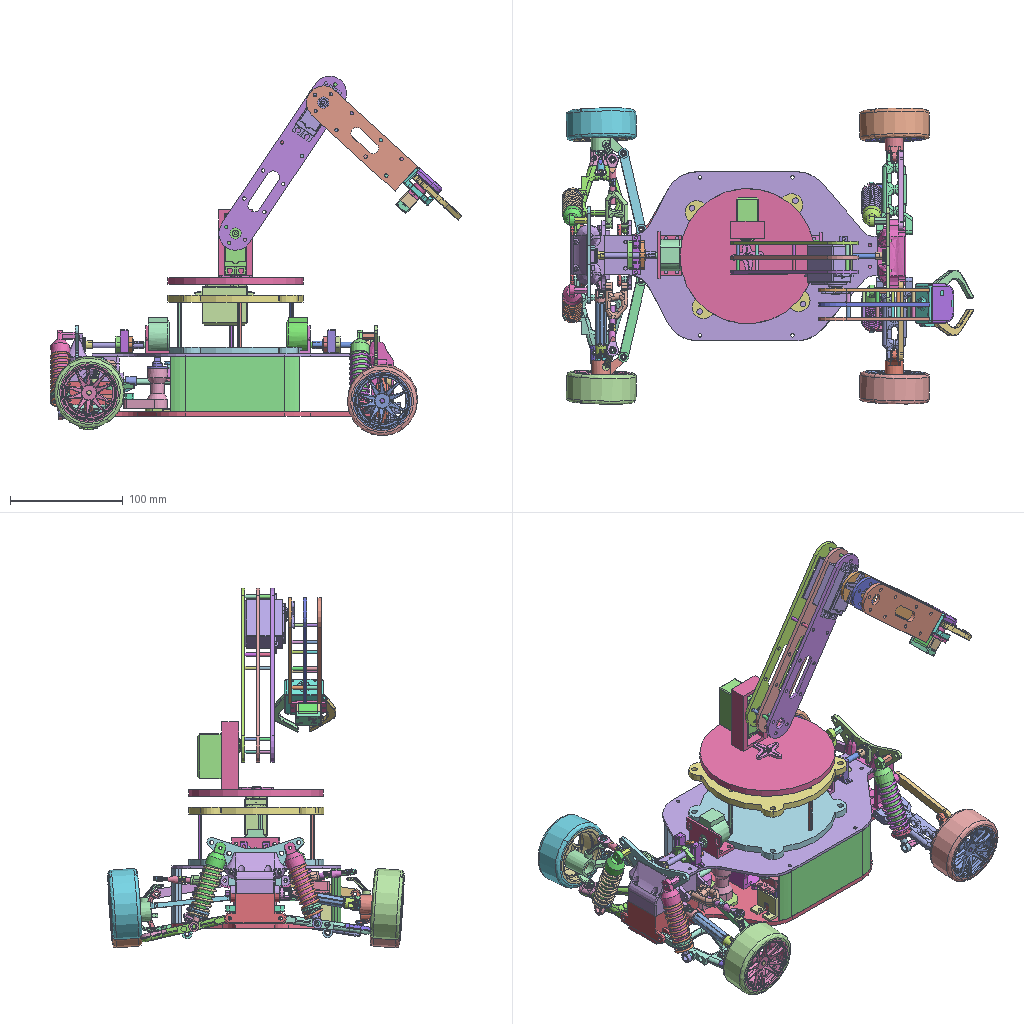Assembly | STEP file | 148 different items | 148 placed | box 365 x 263 x 319 mm
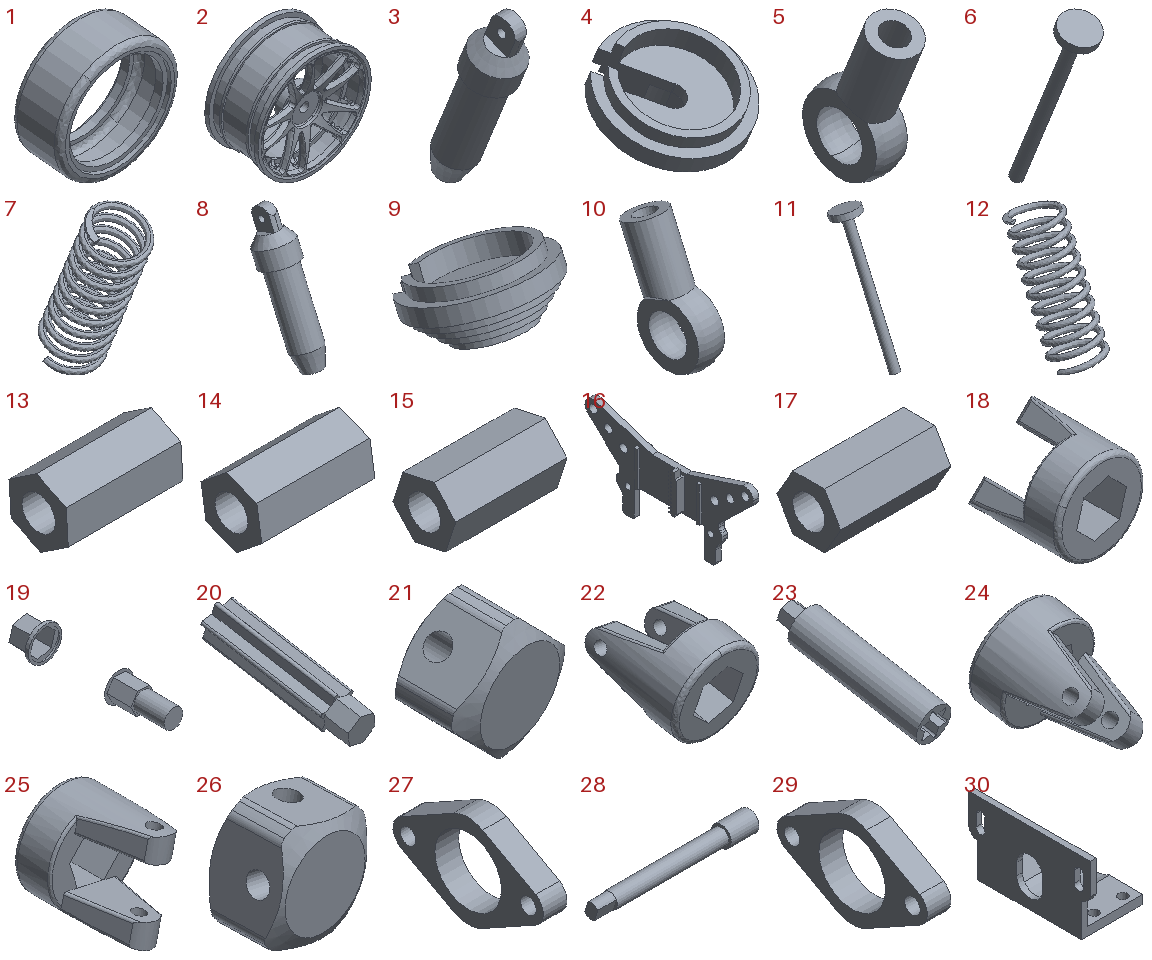Parts list (item | name | quantity | parent item | size | volume):
1 | PNEU | x1 | in JR29_2 | 62.467 x 30.182 x 63.29 mm | 18321 mm3
2 | jante JR29 | x1 | in JR29_2 | 53.113 x 29.9 x 54.23 mm | 11757 mm3
3 | Cut-Extrude2 | x1 | in _115-006 | 16.64 x 30.437 x 60.503 mm | 5800 mm3
4 | Cut-Extrude7 | x1 | in _115-003 | 18 x 17.564 x 12.214 mm | 867.182 mm3
5 | _.0mm Dowel Hole1 | x1 | in _115-001 | 5.5 x 12.284 x 18.097 mm | 294.625 mm3
6 | Revolve1 | x1 | in _115-004 | 9.4 x 23.118 x 45.968 mm | 456.882 mm3
7 | Ci_cie powierzchni_3 | x1 | in _120-006 | 18 x 31.651 x 49.627 mm | 1562 mm3
8 | Cut-Extrude2 | x1 | in _115-006 | 16.64 x 32.155 x 59.897 mm | 5800 mm3
9 | Cut-Extrude7 | x1 | in _115-003 | 18 x 17.404 x 12.495 mm | 867.182 mm3
10 | _.0mm Dowel Hole1 | x1 | in _115-001 | 5.5 x 12.651 x 18.014 mm | 294.626 mm3
11 | Revolve1 | x1 | in _115-004 | 9.4 x 24.478 x 45.558 mm | 456.882 mm3
12 | Ci_cie powierzchni_3 | x1 | in _120-006 | 18 x 34.556 x 45.056 mm | 1562 mm3
13 | Dodanie-wyci_gni_cie1_8 | x1 | in dystanse amortyzatora | 11 x 5.689 x 6.325 mm | 198.638 mm3
14 | Dodanie-wyci_gni_cie1_8 | x1 | in dystanse amortyzatora | 11 x 5.919 x 6.26 mm | 198.638 mm3
15 | Dodanie-wyci_gni_cie1_8 | x1 | in dystanse amortyzatora | 11 x 6.193 x 6.041 mm | 198.638 mm3
16 | Dodanie-wyci_gni_cie4_3 | x1 | in _400-008 | 8.15 x 85.559 x 42.443 mm | 4763 mm3
17 | Dodanie-wyci_gni_cie1_8 | x1 | in dystanse amortyzatora | 11 x 6.339 x 5.502 mm | 198.638 mm3
18 | Wytnij-wyci_gni_cie1_8 | x1 | in _151-004 | 10.019 x 11.057 x 10.028 mm | 351.853 mm3
19 | Przeci_cie1[1] | x1 | in _151-002 | 7.004 x 31.35 x 7.006 mm | 710.625 mm3
20 | Dodanie-wyci_gni_cie2_4 | x1 | in _151-005 | 7.193 x 30.668 x 11.467 mm | 797.649 mm3
21 | Wytnij-wyci_gni_cie2_4 | x1 | in _151-003 | 6.818 x 4.485 x 6.828 mm | 88.126 mm3
22 | Wytnij-wyci_gni_cie1_8 | x1 | in _151-004 | 10.007 x 11.818 x 10.415 mm | 351.853 mm3
23 | Dodanie-wyci_gni_cie3 | x1 | in _151-006 | 9.523 x 41.689 x 15.416 mm | 1560 mm3
24 | Wytnij-wyci_gni_cie1_8 | x1 | in _151-004 | 10.002 x 12.22 x 10.913 mm | 351.853 mm3
25 | Wytnij-wyci_gni_cie1_8 | x1 | in _151-004 | 10 x 11 x 10 mm | 351.853 mm3
26 | Wytnij-wyci_gni_cie2_4 | x1 | in _151-003 | 5.85 x 4.13 x 6.16 mm | 88.126 mm3
27 | Dodanie-wyci_gni_cie1_6 | x1 | in _400-005 | 3.95 x 25 x 15.427 mm | 542.296 mm3
28 | Dodanie-wyci_gni_cie4_1 | x1 | in _400-003 | 51 x 6.5 x 6.5 mm | 982.022 mm3
29 | Dodanie-wyci_gni_cie1_6 | x1 | in _400-005 | 3.95 x 25 x 15.427 mm | 542.296 mm3
30 | Wytnij-wyci_gni_cie6_2 | x1 | in _400-002 | 21.259 x 42 x 25 mm | 3415 mm3
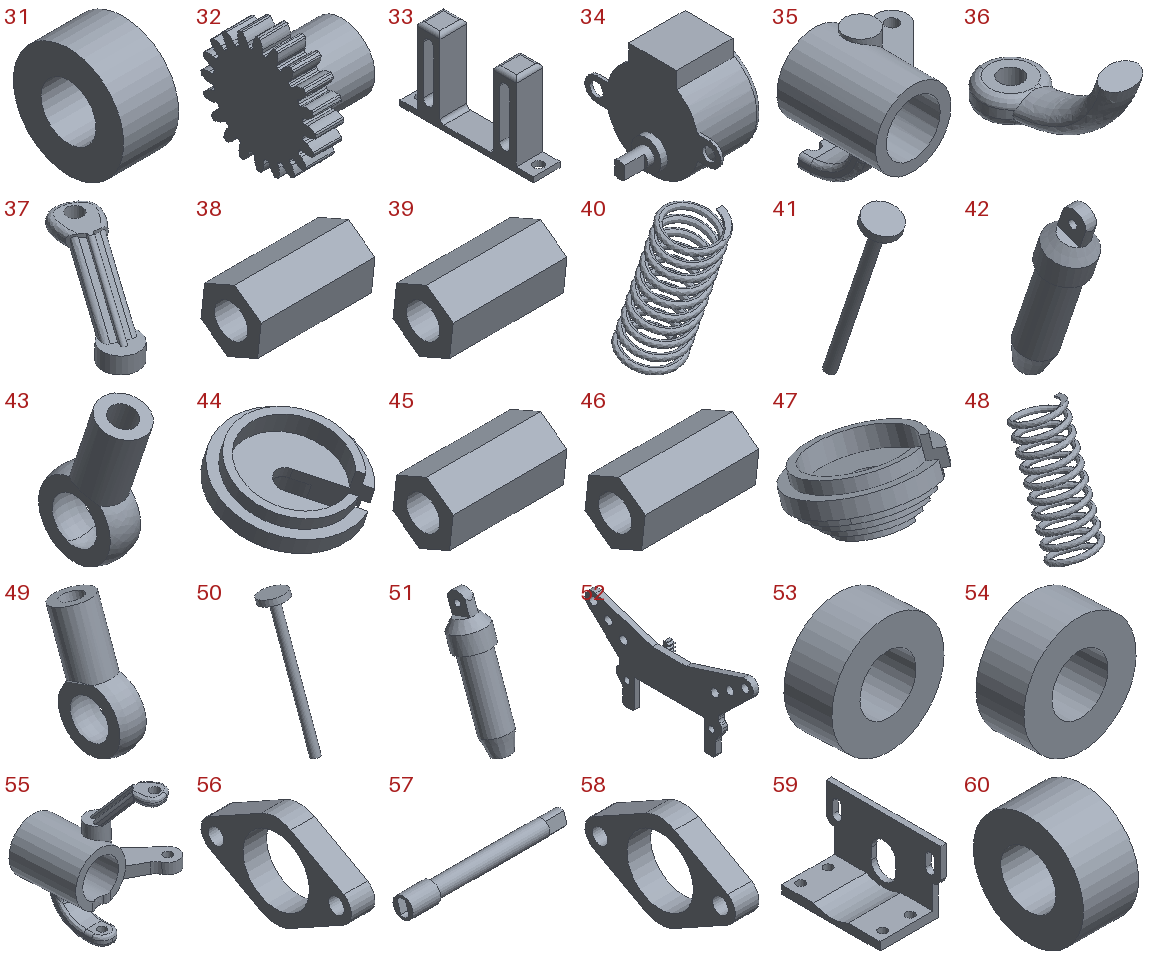31 | Dodanie-wyci_gni_cie1_7 | x1 | in _400-007 | 5 x 10 x 10 mm | 294.524 mm3
32 | Wytnij-wyci_gni_cie1_7 | x1 | in _400-006 | 9 x 12.32 x 12.32 mm | 463.728 mm3
33 | Wytnij-wyci_gni_cie4 | x1 | in _400-004 | 7 x 35 x 21.379 mm | 1461 mm3
34 | Wytnij-wyci_gni_cie1_6 | x1 | in _400-001 | 29 x 41 x 31 mm | 12849 mm3
35 | Zaokr_glenie5_1 | x1 | in _140-001-lewa | 32.058 x 28.351 x 26.679 mm | 3338 mm3
36 | Wytnij-wyci_gni_cie10 | x1 | in _140-001-lewa | 7.005 x 17.81 x 9.853 mm | 233.546 mm3
37 | - | x1 | in _140-001-lewa | 12.902 x 21.037 x 15.015 mm | 400.583 mm3
38 | Dodanie-wyci_gni_cie1_8 | x1 | in dystanse amortyzatora | 11 x 5.805 x 6.301 mm | 198.638 mm3
39 | Dodanie-wyci_gni_cie1_8 | x1 | in dystanse amortyzatora | 11 x 5.805 x 6.301 mm | 198.638 mm3
40 | Ci_cie powierzchni_3 | x1 | in _120-006 | 18 x 31.486 x 45.126 mm | 1562 mm3
41 | Revolve1 | x1 | in _115-004 | 9.4 x 20.928 x 46.51 mm | 456.882 mm3
42 | Cut-Extrude2 | x1 | in _115-006 | 16.64 x 27.67 x 61.336 mm | 5800 mm3
43 | _.0mm Dowel Hole1 | x1 | in _115-001 | 5.5 x 11.691 x 18.199 mm | 294.626 mm3
44 | Cut-Extrude7 | x1 | in _115-003 | 18 x 17.777 x 11.744 mm | 867.182 mm3
45 | Dodanie-wyci_gni_cie1_8 | x1 | in dystanse amortyzatora | 11 x 5.805 x 6.301 mm | 198.638 mm3
46 | Dodanie-wyci_gni_cie1_8 | x1 | in dystanse amortyzatora | 11 x 5.805 x 6.301 mm | 198.638 mm3
47 | Cut-Extrude7 | x1 | in _115-003 | 18 x 17.702 x 11.925 mm | 867.182 mm3
48 | Ci_cie powierzchni_3 | x1 | in _120-006 | 18 x 30.619 x 49.676 mm | 1562 mm3
49 | _.0mm Dowel Hole1 | x1 | in _115-001 | 5.5 x 11.917 x 18.165 mm | 294.625 mm3
50 | Revolve1 | x1 | in _115-004 | 9.4 x 21.762 x 46.32 mm | 456.882 mm3
51 | Cut-Extrude2 | x1 | in _115-006 | 16.64 x 28.724 x 61.039 mm | 5800 mm3
52 | Zapas-_111-007-1 | x1 | in _400-009.1 | 6.85 x 85.559 x 42.443 mm | 4712 mm3
53 | Dodanie-wyci_gni_cie1_3 | x1 | in _140-002 | 12.066 x 5.461 x 12.174 mm | 424.115 mm3
54 | Dodanie-wyci_gni_cie1_3 | x1 | in _140-002 | 12.066 x 5.461 x 12.174 mm | 424.115 mm3
55 | Zaokr_glenie5 | x1 | in _140-001-prawa | 32.405 x 33.388 x 41.862 mm | 3783 mm3
56 | Dodanie-wyci_gni_cie1_6 | x1 | in _400-005 | 3.95 x 25 x 15.427 mm | 542.296 mm3
57 | Dodanie-wyci_gni_cie4_1 | x1 | in _400-003 | 51 x 6.5 x 6.5 mm | 982.022 mm3
58 | Dodanie-wyci_gni_cie1_6 | x1 | in _400-005 | 3.95 x 25 x 15.427 mm | 542.296 mm3
59 | Wytnij-wyci_gni_cie6_2 | x1 | in _400-002 | 21.259 x 42 x 25 mm | 3415 mm3
60 | Dodanie-wyci_gni_cie1_7 | x1 | in _400-007 | 5 x 10 x 10 mm | 294.524 mm3
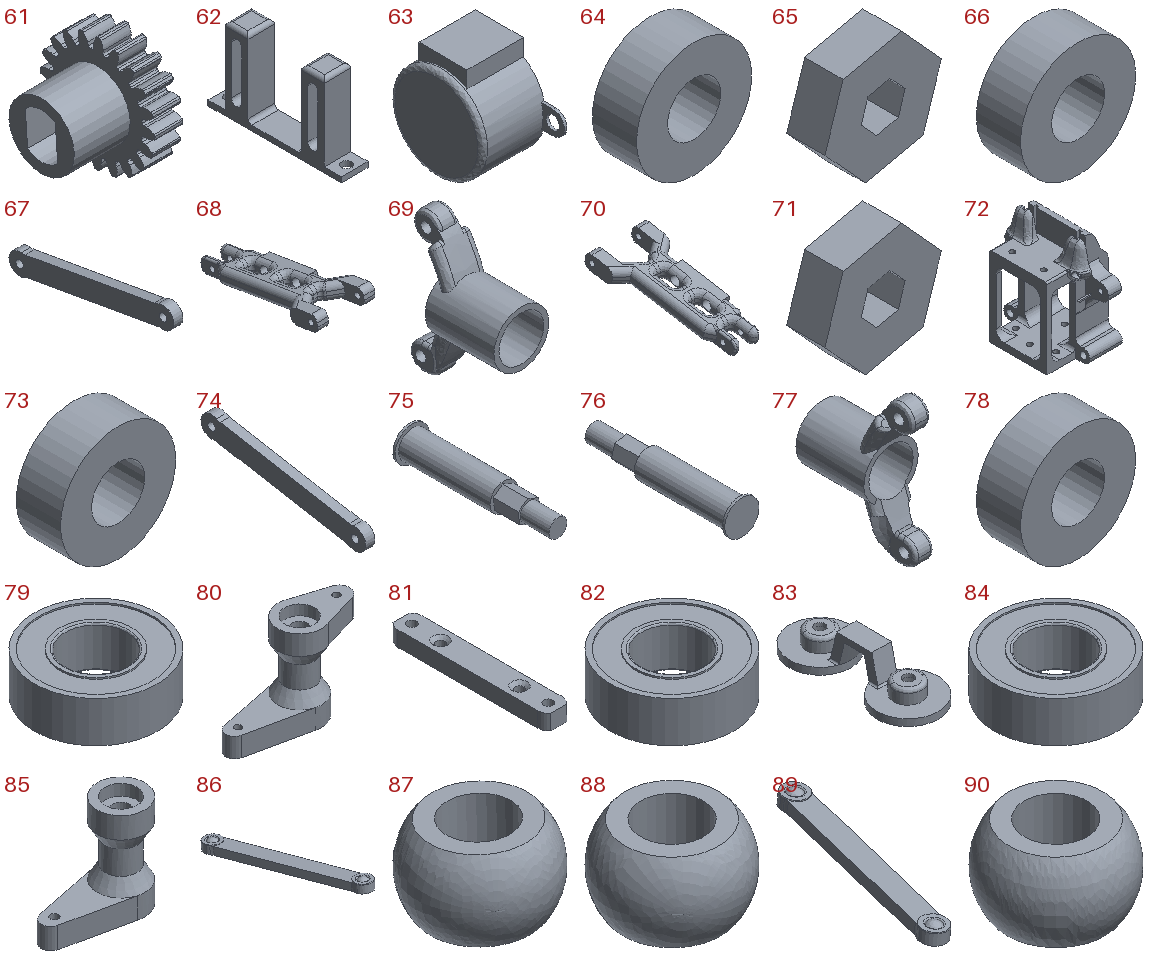61 | Wytnij-wyci_gni_cie1_7 | x1 | in _400-006 | 9 x 12.32 x 12.32 mm | 463.728 mm3
62 | Wytnij-wyci_gni_cie4 | x1 | in _400-004 | 7 x 35 x 21.379 mm | 1461 mm3
63 | Wytnij-wyci_gni_cie1_6 | x1 | in _400-001 | 29 x 41 x 31 mm | 12849 mm3
64 | Dodanie-wyci_gni_cie1_4 | x1 | in _200-006 | 13 x 5.005 x 13.002 mm | 522.29 mm3
65 | Dodanie-wyci_gni_cie1_5 | x1 | in _150-003 | 13.678 x 4.505 x 13.341 mm | 491.011 mm3
66 | Dodanie-wyci_gni_cie1_4 | x1 | in _200-006 | 13 x 5.005 x 13.002 mm | 522.29 mm3
67 | Dodanie-wyci_gni_cie2_2 | x1 | in _200-003 | 4 x 70.047 x 19.826 mm | 2190 mm3
68 | Wytnij-wyci_gni_cie2_2 | x1 | in _200-002 | 32 x 74.835 x 19.276 mm | 7840 mm3
69 | Wytnij-wyci_gni_cie8 | x1 | in _200-004 | 16 x 29.947 x 40.939 mm | 2434 mm3
70 | Wytnij-wyci_gni_cie2_2 | x1 | in _200-002 | 32 x 74.835 x 19.276 mm | 7840 mm3
71 | Dodanie-wyci_gni_cie1_5 | x1 | in _150-003 | 13.678 x 4.505 x 13.341 mm | 491.011 mm3
72 | Lustro3 | x1 | in _200-001 | 37.601 x 63.709 x 62.254 mm | 29031 mm3
73 | Dodanie-wyci_gni_cie1_4 | x1 | in _200-006 | 13 x 5.005 x 13.002 mm | 522.29 mm3
74 | Dodanie-wyci_gni_cie2_2 | x1 | in _200-003 | 4 x 70.047 x 19.826 mm | 2190 mm3
75 | Dodanie-wyci_gni_cie4_2 | x1 | in _200-005 | 7.5 x 32.302 x 7.5 mm | 765.405 mm3
76 | Dodanie-wyci_gni_cie4_2 | x1 | in _200-005 | 7.5 x 32.302 x 7.5 mm | 765.405 mm3
77 | Wytnij-wyci_gni_cie8 | x1 | in _200-004 | 16 x 29.947 x 40.939 mm | 2434 mm3
78 | Dodanie-wyci_gni_cie1_4 | x1 | in _200-006 | 13 x 5.005 x 13.002 mm | 522.29 mm3
79 | Zapas-OpenRC Truggy HSPr v2. v55-1 | x1 | in _131-003 | 12 x 12 x 4 mm | 322.133 mm3
80 | Dodanie-wyci_gni_cie2 | x1 | in _131-002 | 50.275 x 17.999 x 35 mm | 7787 mm3
81 | Wytnij-wyci_gni_cie1_1 | x1 | in _131-006 | 8 x 52 x 5 mm | 1902 mm3
82 | Zapas-OpenRC Truggy HSPr v2. v55-1 | x1 | in _131-003 | 12 x 12 x 4 mm | 322.133 mm3
83 | Wytnij-wyci_gni_cie3_1 | x1 | in _131-008 | 18.204 x 43.999 x 10 mm | 1454 mm3
84 | Zapas-OpenRC Truggy HSPr v2. v55-1 | x1 | in _131-003 | 12 x 12 x 4 mm | 322.133 mm3
85 | Dodanie-wyci_gni_cie1_2 | x1 | in _131-005 | 38.999 x 17.999 x 35 mm | 6844 mm3
86 | Zaokr_glenie2 | x1 | in _131-007 | 24.844 x 77.037 x 13.475 mm | 2577 mm3
87 | Wytnij-wyci_gni_cie1_2 | x1 | in kulka przegubu sterowania | - | 61.693 mm3
88 | Wytnij-wyci_gni_cie1_2 | x1 | in kulka przegubu sterowania | - | 61.693 mm3
89 | Zaokr_glenie2 | x1 | in _131-007 | 25.053 x 77.12 x 7.399 mm | 2577 mm3
90 | Wytnij-wyci_gni_cie1_2 | x1 | in kulka przegubu sterowania | - | 61.693 mm3
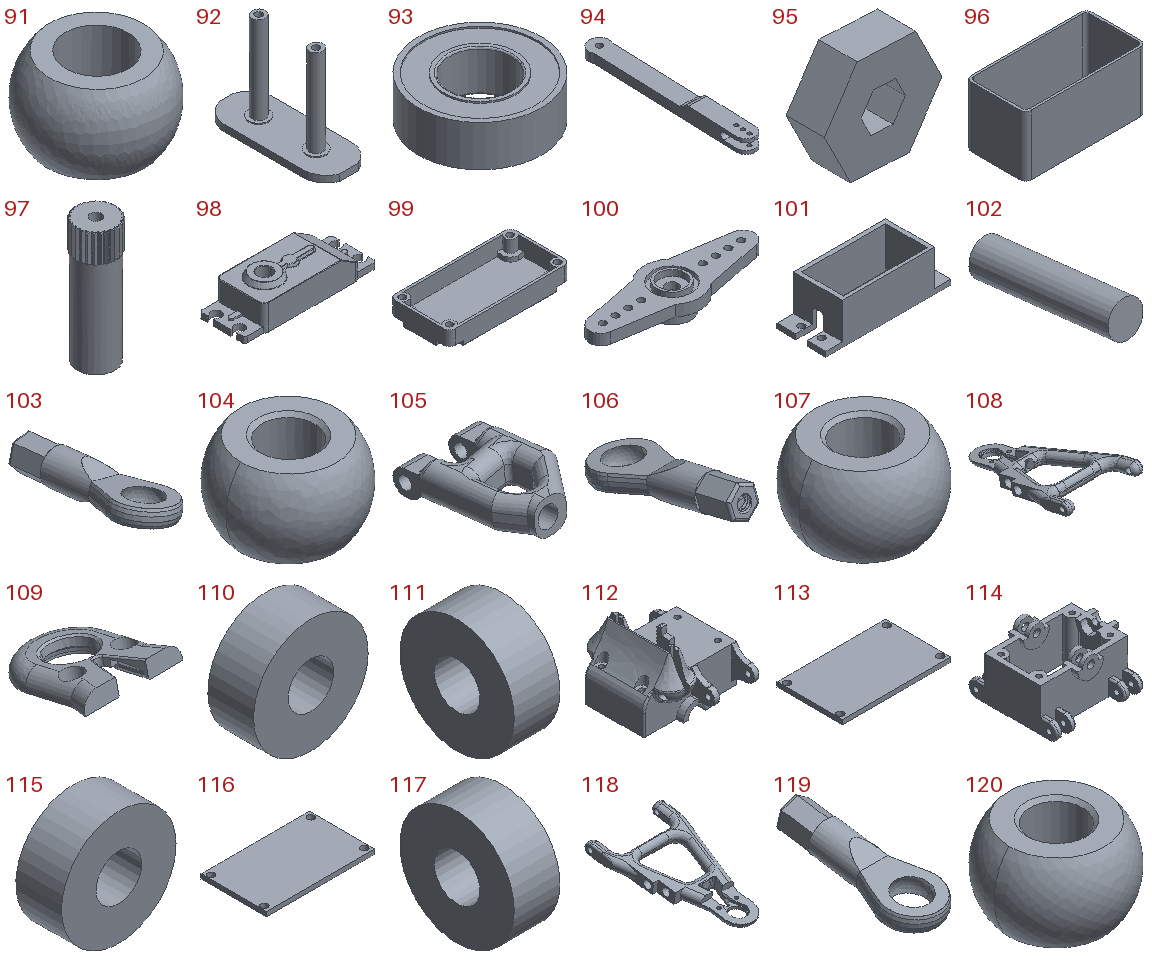91 | Wytnij-wyci_gni_cie1_2 | x1 | in kulka przegubu sterowania | - | 61.693 mm3
92 | Wytnij-wyci_gni_cie1 | x1 | in _131-004 | 21.875 x 55.54 x 43 mm | 5051 mm3
93 | Zapas-OpenRC Truggy HSPr v2. v55-1 | x1 | in _131-003 | 12 x 12 x 4 mm | 322.133 mm3
94 | Wytnij-wyci_gni_cie3 | x1 | in _131-001 | 10.909 x 75.957 x 6 mm | 2529 mm3
95 | Dodanie-wyci_gni_cie1_5 | x1 | in _150-003 | 14.005 x 4.648 x 12.539 mm | 491.011 mm3
96 | Zapas-OpenRC Truggy HSPr v2. v55-3 | x1 | in _132-001 | 41 x 20.4 x 20.5 mm | 1916 mm3
97 | Zapas-OpenRC Truggy HSPr v2. v55-4 | x1 | in _132-001 | 5.799 x 5.767 x 17.5 mm | 382.741 mm3
98 | Zapas-OpenRC Truggy HSPr v2. v55-2 | x1 | in _132-001 | 56 x 20.4 x 13 mm | 9258 mm3
99 | Zapas-OpenRC Truggy HSPr v2. v55-1_1 | x1 | in 99 | - | -
100 | Zapas-OpenRC Truggy HSPr v2. v55-1_2 | x1 | in _132-004 | 38.395 x 12.8 x 5.95 mm | 788.17 mm3
101 | Wytnij-wyci_gni_cie2_3 | x1 | in _132-003 | 60.8 x 23.8 x 20 mm | 5414 mm3
102 | Dodanie-wyci_gni_cie1_1 | x1 | in _114-003 | 5 x 20.432 x 7.194 mm | 392.699 mm3
103 | Zapas-_112-004-1_2 | x1 | in Zapas-_112-004-1 | - | -
104 | Spare ball joint-1 | x1 | in Ball joint-ball | 7 x 7 x 4.494 mm | 116.194 mm3
105 | Wytnij-wyci_gni_cie2 | x1 | in _114-000 | 20 x 33.148 x 11.306 mm | 2601 mm3
106 | Zapas-_112-004-1_2 | x1 | in Zapas-_112-004-1 | - | -
107 | Spare ball joint-1 | x1 | in Ball joint-ball | 7 x 7 x 4.635 mm | 116.194 mm3
108 | Wytnij-wyci_gni_cie6_1 | x1 | in _112-003 | 48 x 82.899 x 24.651 mm | 7377 mm3
109 | - | x1 | in _112-001 | 21.033 x 23.076 x 8.696 mm | 790.702 mm3
110 | Dodanie-wyci_gni_cie1 | x1 | in _111-004 | 10 x 4 x 10 mm | 263.894 mm3
111 | Dodanie-wyci_gni_cie1 | x1 | in _111-004 | 4 x 10 x 10 mm | 263.894 mm3
112 | Wytnij-wyci_gni_cie6 | x1 | in _111-001 | 58 x 61.646 x 42.232 mm | 26812 mm3
113 | Wytnij-wyci_gni_cie8[2] | x1 | in _111-000 | 48 x 29 x 2 mm | 2727 mm3
114 | - | x1 | in _111-000 | 58 x 55 x 32 mm | 19800 mm3
115 | Dodanie-wyci_gni_cie1 | x1 | in _111-004 | 10 x 4 x 10 mm | 263.894 mm3
116 | Zapas-_111-000-1 | x1 | in _111-002 | 48 x 29 x 2 mm | 2727 mm3
117 | Dodanie-wyci_gni_cie1 | x1 | in _111-004 | 4 x 10 x 10 mm | 263.894 mm3
118 | Zaokr_glenie6 | x1 | in _112-002 | 48 x 84.201 x 17.884 mm | 7214 mm3
119 | Zapas-_112-004-1_2 | x1 | in Zapas-_112-004-1 | - | -
120 | Spare ball joint-1 | x1 | in Ball joint-ball | 7 x 7 x 4.494 mm | 116.194 mm3
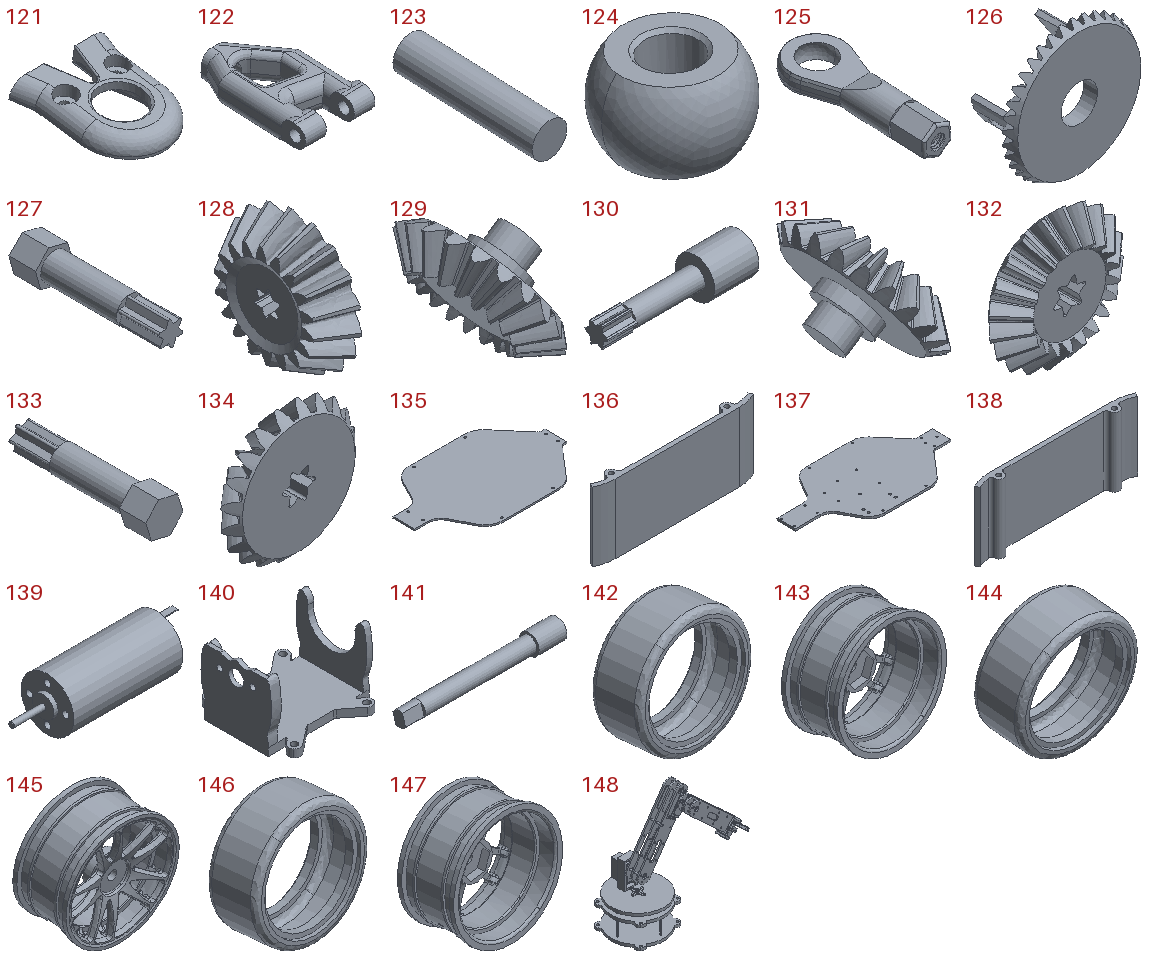121 | - | x1 | in _112-001 | 21.033 x 23.36 x 6.725 mm | 790.702 mm3
122 | Wytnij-wyci_gni_cie2 | x1 | in _114-000 | 20 x 33.189 x 9.079 mm | 2601 mm3
123 | Dodanie-wyci_gni_cie1_1 | x1 | in _114-003 | 5 x 20.198 x 5.864 mm | 392.699 mm3
124 | Spare ball joint-1 | x1 | in Ball joint-ball | 7 x 7 x 4.635 mm | 116.194 mm3
125 | Zapas-_112-004-1_2 | x1 | in Zapas-_112-004-1 | - | -
126 | Zaokr_glenie1 | x1 | in _152-003 | 36.885 x 17.8 x 36.885 mm | 3718 mm3
127 | Zapas-_150-001-1 | x1 | in _151-001 p1 | 5.61 x 21.6 x 5.588 mm | 281.637 mm3
128 | Wytnij-wyci_gni_cie1_3 | x1 | in _150-004(obci_te z_by) | 6 x 19.721 x 19.771 mm | 1055 mm3
129 | Dodanie-wyci_gni_cie2_1 | x1 | in _152-002 | 10.182 x 16.004 x 13.419 mm | 470.763 mm3
130 | Wytnij-wyci_gni_cie5 | x1 | in _150-002 | 29 x 8 x 8 mm | 614.096 mm3
131 | Dodanie-wyci_gni_cie2_1 | x1 | in _152-002 | 10.186 x 16.022 x 13.435 mm | 470.763 mm3
132 | Wytnij-wyci_gni_cie2_1 | x1 | in _152-001 | 15.995 x 3.782 x 15.995 mm | 380.18 mm3
133 | Zapas-_150-001-1 | x1 | in _151-001 p1 | 5.649 x 21.6 x 5.542 mm | 281.637 mm3
134 | Wytnij-wyci_gni_cie2_1 | x1 | in _152-001 | 15.956 x 3.782 x 15.956 mm | 380.18 mm3
135 | Dodanie-wyci_gni_cie2_3 | x1 | in _310-003SLDPRT | 242.308 x 150 x 2.5 mm | 66669 mm3
136 | Zaokr_glenie1_1 | x1 | in _310-004SLDPRT | 114.379 x 8.512 x 49 mm | 19491 mm3
137 | Wytnij-wyci_gni_cie1_5 | x1 | in _310-001 | 296.104 x 150 x 4 mm | 113905 mm3
138 | Zaokr_glenie1_1 | x1 | in _310-004SLDPRT | 114.379 x 8.512 x 49 mm | 19491 mm3
139 | Wytnij-wyci_gni_cie1_4 | x1 | in _153-001 | 75 x 24.6 x 24.6 mm | 24401 mm3
140 | Dodanie-wyci_gni_cie4 | x1 | in _153-003 | 52 x 49.249 x 34.708 mm | 13507 mm3
141 | Dodanie-wyci_gni_cie4_1 | x1 | in _400-003 | 51 x 6.5 x 6.5 mm | 982.022 mm3
142 | PNEU_ Mirror _1 | x1 | in JR29_3_ Mirror | 62.467 x 30.182 x 63.29 mm | 18324 mm3
143 | rim JR29_ Mirror _1 | x1 | in JR29_3_ Mirror | 53.113 x 29.9 x 54.23 mm | 11755 mm3
144 | PNEU | x1 | in JR29_2 | 62.467 x 30.182 x 63.29 mm | 18321 mm3
145 | jante JR29 | x1 | in JR29_2 | 53.113 x 29.9 x 54.23 mm | 11757 mm3
146 | PNEU_ Mirror | x1 | in JR29_2_ Mirror | 62.467 x 30.182 x 63.29 mm | 18324 mm3
147 | rim JR29_ Mirror | x1 | in JR29_2_ Mirror | 53.113 x 29.9 x 54.23 mm | 11755 mm3
148 | Assem1 | x1 | in Wheeled robot | 260.751 x 130.76 x 246.419 mm | 394553 mm3
Placements (level | parent | child | x y z in mm | rotation matrix by rows), first 269 of 321 lines:
1 | root | Frame drive system | 0.0 0.0 0.0 | 1 0 0 0 1 0 0 0 1
2 | Frame drive system | JR29_2 | 0.0 0.0 0.0 | 1 0 0 0 1 0 0 0 1
3 | JR29_2 | PNEU | 0.0 0.0 0.0 | 1 0 0 0 1 0 0 0 1
3 | JR29_2 | jante JR29 | 0.0 0.0 0.0 | 1 0 0 0 1 0 0 0 1
2 | Frame drive system | 000-000_1 | 0.0 0.0 0.0 | 1 0 0 0 1 0 0 0 1
3 | 000-000_1 | _122-000 | 0.0 0.0 0.0 | 1 0 0 0 1 0 0 0 1
4 | _122-000 | _120-000_2 | 0.0 0.0 0.0 | 1 0 0 0 1 0 0 0 1
5 | _120-000_2 | _115-006 | 0.0 0.0 0.0 | 1 0 0 0 1 0 0 0 1
6 | _115-006 | Cut-Extrude2 | 0.0 0.0 0.0 | 1 0 0 0 1 0 0 0 1
5 | _120-000_2 | _115-003 | 0.0 0.0 0.0 | 1 0 0 0 1 0 0 0 1
6 | _115-003 | Cut-Extrude7 | 0.0 0.0 0.0 | 1 0 0 0 1 0 0 0 1
5 | _120-000_2 | _115-001 | 0.0 0.0 0.0 | 1 0 0 0 1 0 0 0 1
6 | _115-001 | _.0mm Dowel Hole1 | 0.0 0.0 0.0 | 1 0 0 0 1 0 0 0 1
5 | _120-000_2 | _115-004 | 0.0 0.0 0.0 | 1 0 0 0 1 0 0 0 1
6 | _115-004 | Revolve1 | 0.0 0.0 0.0 | 1 0 0 0 1 0 0 0 1
5 | _120-000_2 | _120-006 | 0.0 0.0 0.0 | 1 0 0 0 1 0 0 0 1
6 | _120-006 | Ci_cie powierzchni_3 | 0.0 0.0 0.0 | 1 0 0 0 1 0 0 0 1
4 | _122-000 | _120-000_2 | 0.0 0.0 0.0 | 1 0 0 0 1 0 0 0 1
5 | _120-000_2 | _115-006 | 0.0 0.0 0.0 | 1 0 0 0 1 0 0 0 1
6 | _115-006 | Cut-Extrude2 | 0.0 0.0 0.0 | 1 0 0 0 1 0 0 0 1
5 | _120-000_2 | _115-003 | 0.0 0.0 0.0 | 1 0 0 0 1 0 0 0 1
6 | _115-003 | Cut-Extrude7 | 0.0 0.0 0.0 | 1 0 0 0 1 0 0 0 1
5 | _120-000_2 | _115-001 | 0.0 0.0 0.0 | 1 0 0 0 1 0 0 0 1
6 | _115-001 | _.0mm Dowel Hole1 | 0.0 0.0 0.0 | 1 0 0 0 1 0 0 0 1
5 | _120-000_2 | _115-004 | 0.0 0.0 0.0 | 1 0 0 0 1 0 0 0 1
6 | _115-004 | Revolve1 | 0.0 0.0 0.0 | 1 0 0 0 1 0 0 0 1
5 | _120-000_2 | _120-006 | 0.0 0.0 0.0 | 1 0 0 0 1 0 0 0 1
6 | _120-006 | Ci_cie powierzchni_3 | 0.0 0.0 0.0 | 1 0 0 0 1 0 0 0 1
4 | _122-000 | dystanse amortyzatora | 0.0 0.0 0.0 | 1 0 0 0 1 0 0 0 1
5 | dystanse amortyzatora | Dodanie-wyci_gni_cie1_8 | 0.0 0.0 0.0 | 1 0 0 0 1 0 0 0 1
4 | _122-000 | dystanse amortyzatora | 0.0 0.0 0.0 | 1 0 0 0 1 0 0 0 1
5 | dystanse amortyzatora | Dodanie-wyci_gni_cie1_8 | 0.0 0.0 0.0 | 1 0 0 0 1 0 0 0 1
4 | _122-000 | dystanse amortyzatora | 0.0 0.0 0.0 | 1 0 0 0 1 0 0 0 1
5 | dystanse amortyzatora | Dodanie-wyci_gni_cie1_8 | 0.0 0.0 0.0 | 1 0 0 0 1 0 0 0 1
4 | _122-000 | _400-008 | 0.0 0.0 0.0 | 1 0 0 0 1 0 0 0 1
5 | _400-008 | Dodanie-wyci_gni_cie4_3 | 0.0 0.0 0.0 | 1 0 0 0 1 0 0 0 1
4 | _122-000 | dystanse amortyzatora | 0.0 0.0 0.0 | 1 0 0 0 1 0 0 0 1
5 | dystanse amortyzatora | Dodanie-wyci_gni_cie1_8 | 0.0 0.0 0.0 | 1 0 0 0 1 0 0 0 1
3 | 000-000_1 | _151-000 | 0.0 0.0 0.0 | 1 0 0 0 1 0 0 0 1
4 | _151-000 | _151-004 | 0.0 0.0 0.0 | 1 0 0 0 1 0 0 0 1
5 | _151-004 | Wytnij-wyci_gni_cie1_8 | 0.0 0.0 0.0 | 1 0 0 0 1 0 0 0 1
4 | _151-000 | _151-002 | 0.0 0.0 0.0 | 1 0 0 0 1 0 0 0 1
5 | _151-002 | Przeci_cie1[1] | 0.0 0.0 0.0 | 1 0 0 0 1 0 0 0 1
4 | _151-000 | _151-005 | 0.0 0.0 0.0 | 1 0 0 0 1 0 0 0 1
5 | _151-005 | Dodanie-wyci_gni_cie2_4 | 0.0 0.0 0.0 | 1 0 0 0 1 0 0 0 1
4 | _151-000 | _151-003 | 0.0 0.0 0.0 | 1 0 0 0 1 0 0 0 1
5 | _151-003 | Wytnij-wyci_gni_cie2_4 | 0.0 0.0 0.0 | 1 0 0 0 1 0 0 0 1
4 | _151-000 | _151-004 | 0.0 0.0 0.0 | 1 0 0 0 1 0 0 0 1
5 | _151-004 | Wytnij-wyci_gni_cie1_8 | 0.0 0.0 0.0 | 1 0 0 0 1 0 0 0 1
4 | _151-000 | _151-006 | 0.0 0.0 0.0 | 1 0 0 0 1 0 0 0 1
5 | _151-006 | Dodanie-wyci_gni_cie3 | 0.0 0.0 0.0 | 1 0 0 0 1 0 0 0 1
4 | _151-000 | _151-004 | 0.0 0.0 0.0 | 1 0 0 0 1 0 0 0 1
5 | _151-004 | Wytnij-wyci_gni_cie1_8 | 0.0 0.0 0.0 | 1 0 0 0 1 0 0 0 1
4 | _151-000 | _151-004 | 0.0 0.0 0.0 | 1 0 0 0 1 0 0 0 1
5 | _151-004 | Wytnij-wyci_gni_cie1_8 | 0.0 0.0 0.0 | 1 0 0 0 1 0 0 0 1
4 | _151-000 | _151-003 | 0.0 0.0 0.0 | 1 0 0 0 1 0 0 0 1
5 | _151-003 | Wytnij-wyci_gni_cie2_4 | 0.0 0.0 0.0 | 1 0 0 0 1 0 0 0 1
3 | 000-000_1 | _400-000 | 0.0 0.0 0.0 | 1 0 0 0 1 0 0 0 1
4 | _400-000 | _400-005 | 0.0 0.0 0.0 | 1 0 0 0 1 0 0 0 1
5 | _400-005 | Dodanie-wyci_gni_cie1_6 | 0.0 0.0 0.0 | 1 0 0 0 1 0 0 0 1
4 | _400-000 | _400-003 | 0.0 0.0 0.0 | 1 0 0 0 1 0 0 0 1
5 | _400-003 | Dodanie-wyci_gni_cie4_1 | 0.0 0.0 0.0 | 1 0 0 0 1 0 0 0 1
4 | _400-000 | _400-005 | 0.0 0.0 0.0 | 1 0 0 0 1 0 0 0 1
5 | _400-005 | Dodanie-wyci_gni_cie1_6 | 0.0 0.0 0.0 | 1 0 0 0 1 0 0 0 1
4 | _400-000 | _400-002 | 0.0 0.0 0.0 | 1 0 0 0 1 0 0 0 1
5 | _400-002 | Wytnij-wyci_gni_cie6_2 | 0.0 0.0 0.0 | 1 0 0 0 1 0 0 0 1
4 | _400-000 | _400-007 | 0.0 0.0 0.0 | 1 0 0 0 1 0 0 0 1
5 | _400-007 | Dodanie-wyci_gni_cie1_7 | 0.0 0.0 0.0 | 1 0 0 0 1 0 0 0 1
4 | _400-000 | _400-006 | 0.0 0.0 0.0 | 1 0 0 0 1 0 0 0 1
5 | _400-006 | Wytnij-wyci_gni_cie1_7 | 0.0 0.0 0.0 | 1 0 0 0 1 0 0 0 1
4 | _400-000 | _400-004 | 0.0 0.0 0.0 | 1 0 0 0 1 0 0 0 1
5 | _400-004 | Wytnij-wyci_gni_cie4 | 0.0 0.0 0.0 | 1 0 0 0 1 0 0 0 1
4 | _400-000 | _400-001 | 0.0 0.0 0.0 | 1 0 0 0 1 0 0 0 1
5 | _400-001 | Wytnij-wyci_gni_cie1_6 | 0.0 0.0 0.0 | 1 0 0 0 1 0 0 0 1
3 | 000-000_1 | _140-001-lewa | 0.0 0.0 0.0 | 1 0 0 0 1 0 0 0 1
4 | _140-001-lewa | Zaokr_glenie5_1 | 0.0 0.0 0.0 | 1 0 0 0 1 0 0 0 1
4 | _140-001-lewa | Wytnij-wyci_gni_cie10 | 0.0 0.0 0.0 | 1 0 0 0 1 0 0 0 1
4 | _140-001-lewa | subassembly 2 | 0.0 0.0 0.0 | 1 0 0 0 1 0 0 0 1
3 | 000-000_1 | _121-000 | 0.0 0.0 0.0 | 1 0 0 0 1 0 0 0 1
4 | _121-000 | dystanse amortyzatora | 0.0 0.0 0.0 | 1 0 0 0 1 0 0 0 1
5 | dystanse amortyzatora | Dodanie-wyci_gni_cie1_8 | 0.0 0.0 0.0 | 1 0 0 0 1 0 0 0 1
4 | _121-000 | dystanse amortyzatora | 0.0 0.0 0.0 | 1 0 0 0 1 0 0 0 1
5 | dystanse amortyzatora | Dodanie-wyci_gni_cie1_8 | 0.0 0.0 0.0 | 1 0 0 0 1 0 0 0 1
4 | _121-000 | _120-000 | 0.0 0.0 0.0 | 1 0 0 0 1 0 0 0 1
5 | _120-000 | _120-006 | 0.0 0.0 0.0 | 1 0 0 0 1 0 0 0 1
6 | _120-006 | Ci_cie powierzchni_3 | 0.0 0.0 0.0 | 1 0 0 0 1 0 0 0 1
5 | _120-000 | _115-004 | 0.0 0.0 0.0 | 1 0 0 0 1 0 0 0 1
6 | _115-004 | Revolve1 | 0.0 0.0 0.0 | 1 0 0 0 1 0 0 0 1
5 | _120-000 | _115-006 | 0.0 0.0 0.0 | 1 0 0 0 1 0 0 0 1
6 | _115-006 | Cut-Extrude2 | 0.0 0.0 0.0 | 1 0 0 0 1 0 0 0 1
5 | _120-000 | _115-001 | 0.0 0.0 0.0 | 1 0 0 0 1 0 0 0 1
6 | _115-001 | _.0mm Dowel Hole1 | 0.0 0.0 0.0 | 1 0 0 0 1 0 0 0 1
5 | _120-000 | _115-003 | 0.0 0.0 0.0 | 1 0 0 0 1 0 0 0 1
6 | _115-003 | Cut-Extrude7 | 0.0 0.0 0.0 | 1 0 0 0 1 0 0 0 1
4 | _121-000 | dystanse amortyzatora | 0.0 0.0 0.0 | 1 0 0 0 1 0 0 0 1
5 | dystanse amortyzatora | Dodanie-wyci_gni_cie1_8 | 0.0 0.0 0.0 | 1 0 0 0 1 0 0 0 1
4 | _121-000 | dystanse amortyzatora | 0.0 0.0 0.0 | 1 0 0 0 1 0 0 0 1
5 | dystanse amortyzatora | Dodanie-wyci_gni_cie1_8 | 0.0 0.0 0.0 | 1 0 0 0 1 0 0 0 1
4 | _121-000 | _120-000_1 | 0.0 0.0 0.0 | 1 0 0 0 1 0 0 0 1
5 | _120-000_1 | _115-003 | 0.0 0.0 0.0 | 1 0 0 0 1 0 0 0 1
6 | _115-003 | Cut-Extrude7 | 0.0 0.0 0.0 | 1 0 0 0 1 0 0 0 1
5 | _120-000_1 | _120-006 | 0.0 0.0 0.0 | 1 0 0 0 1 0 0 0 1
6 | _120-006 | Ci_cie powierzchni_3 | 0.0 0.0 0.0 | 1 0 0 0 1 0 0 0 1
5 | _120-000_1 | _115-001 | 0.0 0.0 0.0 | 1 0 0 0 1 0 0 0 1
6 | _115-001 | _.0mm Dowel Hole1 | 0.0 0.0 0.0 | 1 0 0 0 1 0 0 0 1
5 | _120-000_1 | _115-004 | 0.0 0.0 0.0 | 1 0 0 0 1 0 0 0 1
6 | _115-004 | Revolve1 | 0.0 0.0 0.0 | 1 0 0 0 1 0 0 0 1
5 | _120-000_1 | _115-006 | 0.0 0.0 0.0 | 1 0 0 0 1 0 0 0 1
6 | _115-006 | Cut-Extrude2 | 0.0 0.0 0.0 | 1 0 0 0 1 0 0 0 1
4 | _121-000 | _400-009.1 | 0.0 0.0 0.0 | 1 0 0 0 1 0 0 0 1
5 | _400-009.1 | Zapas-_111-007-1 | 0.0 0.0 0.0 | 1 0 0 0 1 0 0 0 1
3 | 000-000_1 | _140-000 | 0.0 0.0 0.0 | 1 0 0 0 1 0 0 0 1
4 | _140-000 | _140-002 | 0.0 0.0 0.0 | 1 0 0 0 1 0 0 0 1
5 | _140-002 | Dodanie-wyci_gni_cie1_3 | 0.0 0.0 0.0 | 1 0 0 0 1 0 0 0 1
4 | _140-000 | _140-002 | 0.0 0.0 0.0 | 1 0 0 0 1 0 0 0 1
5 | _140-002 | Dodanie-wyci_gni_cie1_3 | 0.0 0.0 0.0 | 1 0 0 0 1 0 0 0 1
4 | _140-000 | _140-001-prawa | 0.0 0.0 0.0 | 1 0 0 0 1 0 0 0 1
5 | _140-001-prawa | Zaokr_glenie5 | 0.0 0.0 0.0 | 1 0 0 0 1 0 0 0 1
3 | 000-000_1 | _400-000 | 0.0 0.0 0.0 | 1 0 0 0 1 0 0 0 1
4 | _400-000 | _400-005 | 0.0 0.0 0.0 | 1 0 0 0 1 0 0 0 1
5 | _400-005 | Dodanie-wyci_gni_cie1_6 | 0.0 0.0 0.0 | 1 0 0 0 1 0 0 0 1
4 | _400-000 | _400-003 | 0.0 0.0 0.0 | 1 0 0 0 1 0 0 0 1
5 | _400-003 | Dodanie-wyci_gni_cie4_1 | 0.0 0.0 0.0 | 1 0 0 0 1 0 0 0 1
4 | _400-000 | _400-005 | 0.0 0.0 0.0 | 1 0 0 0 1 0 0 0 1
5 | _400-005 | Dodanie-wyci_gni_cie1_6 | 0.0 0.0 0.0 | 1 0 0 0 1 0 0 0 1
4 | _400-000 | _400-002 | 0.0 0.0 0.0 | 1 0 0 0 1 0 0 0 1
5 | _400-002 | Wytnij-wyci_gni_cie6_2 | 0.0 0.0 0.0 | 1 0 0 0 1 0 0 0 1
4 | _400-000 | _400-007 | 0.0 0.0 0.0 | 1 0 0 0 1 0 0 0 1
5 | _400-007 | Dodanie-wyci_gni_cie1_7 | 0.0 0.0 0.0 | 1 0 0 0 1 0 0 0 1
4 | _400-000 | _400-006 | 0.0 0.0 0.0 | 1 0 0 0 1 0 0 0 1
5 | _400-006 | Wytnij-wyci_gni_cie1_7 | 0.0 0.0 0.0 | 1 0 0 0 1 0 0 0 1
4 | _400-000 | _400-004 | 0.0 0.0 0.0 | 1 0 0 0 1 0 0 0 1
5 | _400-004 | Wytnij-wyci_gni_cie4 | 0.0 0.0 0.0 | 1 0 0 0 1 0 0 0 1
4 | _400-000 | _400-001 | 0.0 0.0 0.0 | 1 0 0 0 1 0 0 0 1
5 | _400-001 | Wytnij-wyci_gni_cie1_6 | 0.0 0.0 0.0 | 1 0 0 0 1 0 0 0 1
3 | 000-000_1 | _200-000 | 0.0 0.0 0.0 | 1 0 0 0 1 0 0 0 1
4 | _200-000 | _200-006 | 0.0 0.0 0.0 | 1 0 0 0 1 0 0 0 1
5 | _200-006 | Dodanie-wyci_gni_cie1_4 | 0.0 0.0 0.0 | 1 0 0 0 1 0 0 0 1
4 | _200-000 | _150-003 | 0.0 0.0 0.0 | 1 0 0 0 1 0 0 0 1
5 | _150-003 | Dodanie-wyci_gni_cie1_5 | 0.0 0.0 0.0 | 1 0 0 0 1 0 0 0 1
4 | _200-000 | _200-006 | 0.0 0.0 0.0 | 1 0 0 0 1 0 0 0 1
5 | _200-006 | Dodanie-wyci_gni_cie1_4 | 0.0 0.0 0.0 | 1 0 0 0 1 0 0 0 1
4 | _200-000 | _200-003 | 0.0 0.0 0.0 | 1 0 0 0 1 0 0 0 1
5 | _200-003 | Dodanie-wyci_gni_cie2_2 | 0.0 0.0 0.0 | 1 0 0 0 1 0 0 0 1
4 | _200-000 | _200-002 | 0.0 0.0 0.0 | 1 0 0 0 1 0 0 0 1
5 | _200-002 | Wytnij-wyci_gni_cie2_2 | 0.0 0.0 0.0 | 1 0 0 0 1 0 0 0 1
4 | _200-000 | _200-004 | 0.0 0.0 0.0 | 1 0 0 0 1 0 0 0 1
5 | _200-004 | Wytnij-wyci_gni_cie8 | 0.0 0.0 0.0 | 1 0 0 0 1 0 0 0 1
4 | _200-000 | _200-002 | 0.0 0.0 0.0 | 1 0 0 0 1 0 0 0 1
5 | _200-002 | Wytnij-wyci_gni_cie2_2 | 0.0 0.0 0.0 | 1 0 0 0 1 0 0 0 1
4 | _200-000 | _150-003 | 0.0 0.0 0.0 | 1 0 0 0 1 0 0 0 1
5 | _150-003 | Dodanie-wyci_gni_cie1_5 | 0.0 0.0 0.0 | 1 0 0 0 1 0 0 0 1
4 | _200-000 | _200-001 | 0.0 0.0 0.0 | 1 0 0 0 1 0 0 0 1
5 | _200-001 | Lustro3 | 0.0 0.0 0.0 | 1 0 0 0 1 0 0 0 1
4 | _200-000 | _200-006 | 0.0 0.0 0.0 | 1 0 0 0 1 0 0 0 1
5 | _200-006 | Dodanie-wyci_gni_cie1_4 | 0.0 0.0 0.0 | 1 0 0 0 1 0 0 0 1
4 | _200-000 | _200-003 | 0.0 0.0 0.0 | 1 0 0 0 1 0 0 0 1
5 | _200-003 | Dodanie-wyci_gni_cie2_2 | 0.0 0.0 0.0 | 1 0 0 0 1 0 0 0 1
4 | _200-000 | _200-005 | 0.0 0.0 0.0 | 1 0 0 0 1 0 0 0 1
5 | _200-005 | Dodanie-wyci_gni_cie4_2 | 0.0 0.0 0.0 | 1 0 0 0 1 0 0 0 1
4 | _200-000 | _200-005 | 0.0 0.0 0.0 | 1 0 0 0 1 0 0 0 1
5 | _200-005 | Dodanie-wyci_gni_cie4_2 | 0.0 0.0 0.0 | 1 0 0 0 1 0 0 0 1
4 | _200-000 | _200-004 | 0.0 0.0 0.0 | 1 0 0 0 1 0 0 0 1
5 | _200-004 | Wytnij-wyci_gni_cie8 | 0.0 0.0 0.0 | 1 0 0 0 1 0 0 0 1
4 | _200-000 | _200-006 | 0.0 0.0 0.0 | 1 0 0 0 1 0 0 0 1
5 | _200-006 | Dodanie-wyci_gni_cie1_4 | 0.0 0.0 0.0 | 1 0 0 0 1 0 0 0 1
3 | 000-000_1 | _130-000 | 0.0 0.0 0.0 | 1 0 0 0 1 0 0 0 1
4 | _130-000 | _131-003 | 0.0 0.0 0.0 | 1 0 0 0 1 0 0 0 1
5 | _131-003 | Zapas-OpenRC Truggy HSPr v2. v55-1 | 0.0 0.0 0.0 | 1 0 0 0 1 0 0 0 1
4 | _130-000 | _131-002 | 0.0 0.0 0.0 | 1 0 0 0 1 0 0 0 1
5 | _131-002 | Dodanie-wyci_gni_cie2 | 0.0 0.0 0.0 | 1 0 0 0 1 0 0 0 1
4 | _130-000 | _131-006 | 0.0 0.0 0.0 | 1 0 0 0 1 0 0 0 1
5 | _131-006 | Wytnij-wyci_gni_cie1_1 | 0.0 0.0 0.0 | 1 0 0 0 1 0 0 0 1
4 | _130-000 | _131-003 | 0.0 0.0 0.0 | 1 0 0 0 1 0 0 0 1
5 | _131-003 | Zapas-OpenRC Truggy HSPr v2. v55-1 | 0.0 0.0 0.0 | 1 0 0 0 1 0 0 0 1
4 | _130-000 | _131-008 | 0.0 0.0 0.0 | 1 0 0 0 1 0 0 0 1
5 | _131-008 | Wytnij-wyci_gni_cie3_1 | 0.0 0.0 0.0 | 1 0 0 0 1 0 0 0 1
4 | _130-000 | _131-003 | 0.0 0.0 0.0 | 1 0 0 0 1 0 0 0 1
5 | _131-003 | Zapas-OpenRC Truggy HSPr v2. v55-1 | 0.0 0.0 0.0 | 1 0 0 0 1 0 0 0 1
4 | _130-000 | _131-005 | 0.0 0.0 0.0 | 1 0 0 0 1 0 0 0 1
5 | _131-005 | Dodanie-wyci_gni_cie1_2 | 0.0 0.0 0.0 | 1 0 0 0 1 0 0 0 1
4 | _130-000 | _131_1 | 0.0 0.0 0.0 | 1 0 0 0 1 0 0 0 1
5 | _131_1 | _131-007 | 0.0 0.0 0.0 | 1 0 0 0 1 0 0 0 1
6 | _131-007 | Zaokr_glenie2 | 0.0 0.0 0.0 | 1 0 0 0 1 0 0 0 1
5 | _131_1 | kulka przegubu sterowania | 0.0 0.0 0.0 | 1 0 0 0 1 0 0 0 1
6 | kulka przegubu sterowania | Wytnij-wyci_gni_cie1_2 | 0.0 0.0 0.0 | 1 0 0 0 1 0 0 0 1
5 | _131_1 | kulka przegubu sterowania | 0.0 0.0 0.0 | 1 0 0 0 1 0 0 0 1
6 | kulka przegubu sterowania | Wytnij-wyci_gni_cie1_2 | 0.0 0.0 0.0 | 1 0 0 0 1 0 0 0 1
4 | _130-000 | _131 | 0.0 0.0 0.0 | 1 0 0 0 1 0 0 0 1
5 | _131 | _131-007 | 0.0 0.0 0.0 | 1 0 0 0 1 0 0 0 1
6 | _131-007 | Zaokr_glenie2 | 0.0 0.0 0.0 | 1 0 0 0 1 0 0 0 1
5 | _131 | kulka przegubu sterowania | 0.0 0.0 0.0 | 1 0 0 0 1 0 0 0 1
6 | kulka przegubu sterowania | Wytnij-wyci_gni_cie1_2 | 0.0 0.0 0.0 | 1 0 0 0 1 0 0 0 1
5 | _131 | kulka przegubu sterowania | 0.0 0.0 0.0 | 1 0 0 0 1 0 0 0 1
6 | kulka przegubu sterowania | Wytnij-wyci_gni_cie1_2 | 0.0 0.0 0.0 | 1 0 0 0 1 0 0 0 1
4 | _130-000 | _131-004 | 0.0 0.0 0.0 | 1 0 0 0 1 0 0 0 1
5 | _131-004 | Wytnij-wyci_gni_cie1 | 0.0 0.0 0.0 | 1 0 0 0 1 0 0 0 1
4 | _130-000 | _131-003 | 0.0 0.0 0.0 | 1 0 0 0 1 0 0 0 1
5 | _131-003 | Zapas-OpenRC Truggy HSPr v2. v55-1 | 0.0 0.0 0.0 | 1 0 0 0 1 0 0 0 1
4 | _130-000 | _131-001 | 0.0 0.0 0.0 | 1 0 0 0 1 0 0 0 1
5 | _131-001 | Wytnij-wyci_gni_cie3 | 0.0 0.0 0.0 | 1 0 0 0 1 0 0 0 1
3 | 000-000_1 | _150-003 | 0.0 0.0 0.0 | 1 0 0 0 1 0 0 0 1
4 | _150-003 | Dodanie-wyci_gni_cie1_5 | 0.0 0.0 0.0 | 1 0 0 0 1 0 0 0 1
3 | 000-000_1 | _132-000 | 0.0 0.0 0.0 | 1 0 0 0 1 0 0 0 1
4 | _132-000 | _132-001 | 0.0 0.0 0.0 | 1 0 0 0 1 0 0 0 1
5 | _132-001 | Zapas-OpenRC Truggy HSPr v2. v55-3 | 0.0 0.0 0.0 | 1 0 0 0 1 0 0 0 1
5 | _132-001 | Zapas-OpenRC Truggy HSPr v2. v55-4 | 0.0 0.0 0.0 | 1 0 0 0 1 0 0 0 1
5 | _132-001 | Zapas-OpenRC Truggy HSPr v2. v55-2 | 0.0 0.0 0.0 | 1 0 0 0 1 0 0 0 1
5 | _132-001 | Zapas-OpenRC Truggy HSPr v2. v55-1_1 | 0.0 0.0 0.0 | 1 0 0 0 1 0 0 0 1
6 | Zapas-OpenRC Truggy HSPr v2. v55-1_1 | Zapas-OpenRC Truggy HSPr v2. v55-1_1 | 0.0 0.0 0.0 | 1 0 0 0 1 0 0 0 1
4 | _132-000 | _132-004 | 0.0 0.0 0.0 | 1 0 0 0 1 0 0 0 1
5 | _132-004 | Zapas-OpenRC Truggy HSPr v2. v55-1_2 | 0.0 0.0 0.0 | 1 0 0 0 1 0 0 0 1
4 | _132-000 | _132-003 | 0.0 0.0 0.0 | 1 0 0 0 1 0 0 0 1
5 | _132-003 | Wytnij-wyci_gni_cie2_3 | 0.0 0.0 0.0 | 1 0 0 0 1 0 0 0 1
3 | 000-000_1 | _110-000 | 0.0 0.0 0.0 | 1 0 0 0 1 0 0 0 1
4 | _110-000 | _114-000_1 | 0.0 0.0 0.0 | 1 0 0 0 1 0 0 0 1
5 | _114-000_1 | _114-003 | 0.0 0.0 0.0 | 1 0 0 0 1 0 0 0 1
6 | _114-003 | Dodanie-wyci_gni_cie1_1 | 0.0 0.0 0.0 | 1 0 0 0 1 0 0 0 1
5 | _114-000_1 | _114-0002_2 | 0.0 0.0 0.0 | 1 0 0 0 1 0 0 0 1
6 | _114-0002_2 | _112-0041 | 0.0 0.0 0.0 | 1 0 0 0 1 0 0 0 1
7 | _112-0041 | Zapas-_112-004-1 | 0.0 0.0 0.0 | 1 0 0 0 1 0 0 0 1
8 | Zapas-_112-004-1 | Zapas-_112-004-1_2 | 0.0 0.0 0.0 | 1 0 0 0 1 0 0 0 1
6 | _114-0002_2 | Ball joint-ball | 0.0 0.0 0.0 | 1 0 0 0 1 0 0 0 1
7 | Ball joint-ball | Spare ball joint-1 | 0.0 0.0 0.0 | 1 0 0 0 1 0 0 0 1
5 | _114-000_1 | _114-000 | 0.0 0.0 0.0 | 1 0 0 0 1 0 0 0 1
6 | _114-000 | Wytnij-wyci_gni_cie2 | 0.0 0.0 0.0 | 1 0 0 0 1 0 0 0 1
4 | _110-000 | _112-000 | 0.0 0.0 0.0 | 1 0 0 0 1 0 0 0 1
5 | _112-000 | _114-0002 | 0.0 0.0 0.0 | 1 0 0 0 1 0 0 0 1
6 | _114-0002 | _112-0041 | 0.0 0.0 0.0 | 1 0 0 0 1 0 0 0 1
7 | _112-0041 | Zapas-_112-004-1 | 0.0 0.0 0.0 | 1 0 0 0 1 0 0 0 1
8 | Zapas-_112-004-1 | Zapas-_112-004-1_2 | 0.0 0.0 0.0 | 1 0 0 0 1 0 0 0 1
6 | _114-0002 | Ball joint-ball | 0.0 0.0 0.0 | 1 0 0 0 1 0 0 0 1
7 | Ball joint-ball | Spare ball joint-1 | 0.0 0.0 0.0 | 1 0 0 0 1 0 0 0 1
5 | _112-000 | _112-003 | 0.0 0.0 0.0 | 1 0 0 0 1 0 0 0 1
6 | _112-003 | Wytnij-wyci_gni_cie6_1 | 0.0 0.0 0.0 | 1 0 0 0 1 0 0 0 1
5 | _112-000 | _112-001 | 0.0 0.0 0.0 | 1 0 0 0 1 0 0 0 1
6 | _112-001 | subassembly 3 | 0.0 0.0 0.0 | 1 0 0 0 1 0 0 0 1
4 | _110-000 | _111-000_1 | 0.0 0.0 0.0 | 1 0 0 0 1 0 0 0 1
5 | _111-000_1 | _111-004 | 0.0 0.0 0.0 | 1 0 0 0 1 0 0 0 1
6 | _111-004 | Dodanie-wyci_gni_cie1 | 0.0 0.0 0.0 | 1 0 0 0 1 0 0 0 1
5 | _111-000_1 | _111-004 | 0.0 0.0 0.0 | 1 0 0 0 1 0 0 0 1
6 | _111-004 | Dodanie-wyci_gni_cie1 | 0.0 0.0 0.0 | 1 0 0 0 1 0 0 0 1
5 | _111-000_1 | _111-001 | 0.0 0.0 0.0 | 1 0 0 0 1 0 0 0 1
6 | _111-001 | Wytnij-wyci_gni_cie6 | 0.0 0.0 0.0 | 1 0 0 0 1 0 0 0 1
5 | _111-000_1 | _111-000 | 0.0 0.0 0.0 | 1 0 0 0 1 0 0 0 1
6 | _111-000 | Wytnij-wyci_gni_cie8[2] | 0.0 0.0 0.0 | 1 0 0 0 1 0 0 0 1
6 | _111-000 | subassembly 4 | 0.0 0.0 0.0 | 1 0 0 0 1 0 0 0 1
5 | _111-000_1 | _111-004 | 0.0 0.0 0.0 | 1 0 0 0 1 0 0 0 1
6 | _111-004 | Dodanie-wyci_gni_cie1 | 0.0 0.0 0.0 | 1 0 0 0 1 0 0 0 1
5 | _111-000_1 | _111-002 | 0.0 0.0 0.0 | 1 0 0 0 1 0 0 0 1
6 | _111-002 | Zapas-_111-000-1 | 0.0 0.0 0.0 | 1 0 0 0 1 0 0 0 1
5 | _111-000_1 | _111-004 | 0.0 0.0 0.0 | 1 0 0 0 1 0 0 0 1
6 | _111-004 | Dodanie-wyci_gni_cie1 | 0.0 0.0 0.0 | 1 0 0 0 1 0 0 0 1
4 | _110-000 | _113-000 | 0.0 0.0 0.0 | 1 0 0 0 1 0 0 0 1
5 | _113-000 | _112-002 | 0.0 0.0 0.0 | 1 0 0 0 1 0 0 0 1
6 | _112-002 | Zaokr_glenie6 | 0.0 0.0 0.0 | 1 0 0 0 1 0 0 0 1
5 | _113-000 | _114-0002_1 | 0.0 0.0 0.0 | 1 0 0 0 1 0 0 0 1
6 | _114-0002_1 | _112-0041 | 0.0 0.0 0.0 | 1 0 0 0 1 0 0 0 1
7 | _112-0041 | Zapas-_112-004-1 | 0.0 0.0 0.0 | 1 0 0 0 1 0 0 0 1
8 | Zapas-_112-004-1 | Zapas-_112-004-1_2 | 0.0 0.0 0.0 | 1 0 0 0 1 0 0 0 1
6 | _114-0002_1 | Ball joint-ball | 0.0 0.0 0.0 | 1 0 0 0 1 0 0 0 1
7 | Ball joint-ball | Spare ball joint-1 | 0.0 0.0 0.0 | 1 0 0 0 1 0 0 0 1
5 | _113-000 | _112-001 | 0.0 0.0 0.0 | 1 0 0 0 1 0 0 0 1
6 | _112-001 | subassembly 3 | 0.0 0.0 0.0 | 1 0 0 0 1 0 0 0 1
4 | _110-000 | _114-000_2 | 0.0 0.0 0.0 | 1 0 0 0 1 0 0 0 1
5 | _114-000_2 | _114-000 | 0.0 0.0 0.0 | 1 0 0 0 1 0 0 0 1
6 | _114-000 | Wytnij-wyci_gni_cie2 | 0.0 0.0 0.0 | 1 0 0 0 1 0 0 0 1
5 | _114-000_2 | _114-003 | 0.0 0.0 0.0 | 1 0 0 0 1 0 0 0 1
6 | _114-003 | Dodanie-wyci_gni_cie1_1 | 0.0 0.0 0.0 | 1 0 0 0 1 0 0 0 1